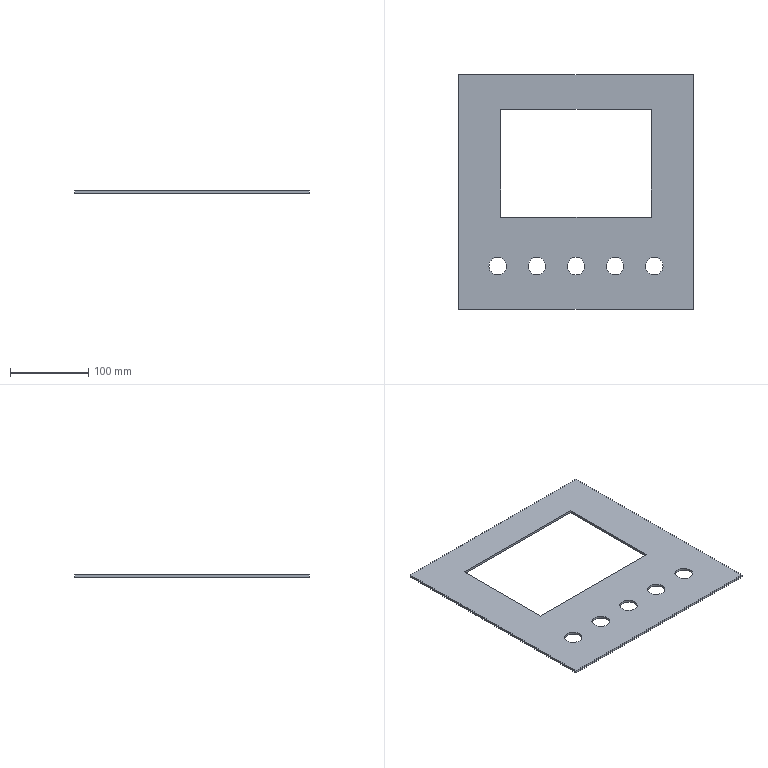Part | SolidWorks | features BaseBody 1 | 1 solid | 20 faces | box 300 x 300 x 3 mm | volume 184548 mm3 | cylinder 10 | plane 10 | commonest cylinder face diameters 22.5 x10
STEP:
#1=CARTESIAN_POINT('',(238.75,55.231,3.));
#2=VERTEX_POINT('',#1);
#3=CARTESIAN_POINT('',(261.25,55.231,3.));
#4=VERTEX_POINT('',#3);
#5=CARTESIAN_POINT('',(250.,55.231,3.));
#6=DIRECTION('',(0.,0.,1.));
#7=DIRECTION('',(-1.,0.,0.));
#8=AXIS2_PLACEMENT_3D('',#5,#6,#7);
#9=CIRCLE('',#8,11.25);
#10=EDGE_CURVE('',#2,#4,#9,.T.);
#11=ORIENTED_EDGE('',*,*,#10,.T.);
#12=CARTESIAN_POINT('',(261.25,55.231,0.));
#13=VERTEX_POINT('',#12);
#14=CARTESIAN_POINT('',(261.25,55.231,3.));
#15=DIRECTION('',(0.,0.,-1.));
#16=VECTOR('',#15,1000.);
#17=LINE('',#14,#16);
#18=EDGE_CURVE('',#4,#13,#17,.T.);
#19=ORIENTED_EDGE('',*,*,#18,.T.);
#20=CARTESIAN_POINT('',(238.75,55.231,0.));
#21=VERTEX_POINT('',#20);
#22=CARTESIAN_POINT('',(250.,55.231,0.));
#23=DIRECTION('',(0.,0.,1.));
#24=DIRECTION('',(-1.,0.,0.));
#25=AXIS2_PLACEMENT_3D('',#22,#23,#24);
#26=CIRCLE('',#25,11.25);
#27=EDGE_CURVE('',#21,#13,#26,.T.);
#28=ORIENTED_EDGE('',*,*,#27,.F.);
#29=CARTESIAN_POINT('',(238.75,55.231,3.));
#30=DIRECTION('',(0.,0.,-1.));
#31=VECTOR('',#30,1000.);
#32=LINE('',#29,#31);
#33=EDGE_CURVE('',#2,#21,#32,.T.);
#34=ORIENTED_EDGE('',*,*,#33,.F.);
#35=EDGE_LOOP('',(#11,#19,#28,#34));
#36=FACE_OUTER_BOUND('',#35,.T.);
#37=CARTESIAN_POINT('',(250.,55.231,3.));
#38=DIRECTION('',(0.,0.,-1.));
#39=DIRECTION('',(-1.,0.,0.));
#40=AXIS2_PLACEMENT_3D('',#37,#38,#39);
#41=CYLINDRICAL_SURFACE('',#40,11.25);
#42=ADVANCED_FACE('',(#36),#41,.F.);
#43=CARTESIAN_POINT('',(188.75,55.231,3.));
#44=VERTEX_POINT('',#43);
#45=CARTESIAN_POINT('',(211.25,55.231,3.));
#46=VERTEX_POINT('',#45);
#47=CARTESIAN_POINT('',(200.,55.231,3.));
#48=DIRECTION('',(0.,0.,1.));
#49=DIRECTION('',(-1.,0.,0.));
#50=AXIS2_PLACEMENT_3D('',#47,#48,#49);
#51=CIRCLE('',#50,11.25);
#52=EDGE_CURVE('',#44,#46,#51,.T.);
#53=ORIENTED_EDGE('',*,*,#52,.T.);
#54=CARTESIAN_POINT('',(211.25,55.231,0.));
#55=VERTEX_POINT('',#54);
#56=CARTESIAN_POINT('',(211.25,55.231,3.));
#57=DIRECTION('',(0.,0.,-1.));
#58=VECTOR('',#57,1000.);
#59=LINE('',#56,#58);
#60=EDGE_CURVE('',#46,#55,#59,.T.);
#61=ORIENTED_EDGE('',*,*,#60,.T.);
#62=CARTESIAN_POINT('',(188.75,55.231,0.));
#63=VERTEX_POINT('',#62);
#64=CARTESIAN_POINT('',(200.,55.231,0.));
#65=DIRECTION('',(0.,0.,1.));
#66=DIRECTION('',(-1.,0.,0.));
#67=AXIS2_PLACEMENT_3D('',#64,#65,#66);
#68=CIRCLE('',#67,11.25);
#69=EDGE_CURVE('',#63,#55,#68,.T.);
#70=ORIENTED_EDGE('',*,*,#69,.F.);
#71=CARTESIAN_POINT('',(188.75,55.231,3.));
#72=DIRECTION('',(0.,0.,-1.));
#73=VECTOR('',#72,1000.);
#74=LINE('',#71,#73);
#75=EDGE_CURVE('',#44,#63,#74,.T.);
#76=ORIENTED_EDGE('',*,*,#75,.F.);
#77=EDGE_LOOP('',(#53,#61,#70,#76));
#78=FACE_OUTER_BOUND('',#77,.T.);
#79=CARTESIAN_POINT('',(200.,55.231,3.));
#80=DIRECTION('',(0.,0.,-1.));
#81=DIRECTION('',(-1.,0.,0.));
#82=AXIS2_PLACEMENT_3D('',#79,#80,#81);
#83=CYLINDRICAL_SURFACE('',#82,11.25);
#84=ADVANCED_FACE('',(#78),#83,.F.);
#85=CARTESIAN_POINT('',(138.75,55.231,3.));
#86=VERTEX_POINT('',#85);
#87=CARTESIAN_POINT('',(161.25,55.231,3.));
#88=VERTEX_POINT('',#87);
#89=CARTESIAN_POINT('',(150.,55.231,3.));
#90=DIRECTION('',(0.,0.,1.));
#91=DIRECTION('',(-1.,0.,0.));
#92=AXIS2_PLACEMENT_3D('',#89,#90,#91);
#93=CIRCLE('',#92,11.25);
#94=EDGE_CURVE('',#86,#88,#93,.T.);
#95=ORIENTED_EDGE('',*,*,#94,.T.);
#96=CARTESIAN_POINT('',(161.25,55.231,0.));
#97=VERTEX_POINT('',#96);
#98=CARTESIAN_POINT('',(161.25,55.231,3.));
#99=DIRECTION('',(0.,0.,-1.));
#100=VECTOR('',#99,1000.);
#101=LINE('',#98,#100);
#102=EDGE_CURVE('',#88,#97,#101,.T.);
#103=ORIENTED_EDGE('',*,*,#102,.T.);
#104=CARTESIAN_POINT('',(138.75,55.231,0.));
#105=VERTEX_POINT('',#104);
#106=CARTESIAN_POINT('',(150.,55.231,0.));
#107=DIRECTION('',(0.,0.,1.));
#108=DIRECTION('',(-1.,0.,0.));
#109=AXIS2_PLACEMENT_3D('',#106,#107,#108);
#110=CIRCLE('',#109,11.25);
#111=EDGE_CURVE('',#105,#97,#110,.T.);
#112=ORIENTED_EDGE('',*,*,#111,.F.);
#113=CARTESIAN_POINT('',(138.75,55.231,3.));
#114=DIRECTION('',(0.,0.,-1.));
#115=VECTOR('',#114,1000.);
#116=LINE('',#113,#115);
#117=EDGE_CURVE('',#86,#105,#116,.T.);
#118=ORIENTED_EDGE('',*,*,#117,.F.);
#119=EDGE_LOOP('',(#95,#103,#112,#118));
#120=FACE_OUTER_BOUND('',#119,.T.);
#121=CARTESIAN_POINT('',(150.,55.231,3.));
#122=DIRECTION('',(0.,0.,-1.));
#123=DIRECTION('',(-1.,0.,0.));
#124=AXIS2_PLACEMENT_3D('',#121,#122,#123);
#125=CYLINDRICAL_SURFACE('',#124,11.25);
#126=ADVANCED_FACE('',(#120),#125,.F.);
#127=CARTESIAN_POINT('',(88.75,55.231,3.));
#128=VERTEX_POINT('',#127);
#129=CARTESIAN_POINT('',(111.25,55.231,3.));
#130=VERTEX_POINT('',#129);
#131=CARTESIAN_POINT('',(100.,55.231,3.));
#132=DIRECTION('',(0.,0.,1.));
#133=DIRECTION('',(-1.,0.,0.));
#134=AXIS2_PLACEMENT_3D('',#131,#132,#133);
#135=CIRCLE('',#134,11.25);
#136=EDGE_CURVE('',#128,#130,#135,.T.);
#137=ORIENTED_EDGE('',*,*,#136,.T.);
#138=CARTESIAN_POINT('',(111.25,55.231,0.));
#139=VERTEX_POINT('',#138);
#140=CARTESIAN_POINT('',(111.25,55.231,3.));
#141=DIRECTION('',(0.,0.,-1.));
#142=VECTOR('',#141,1000.);
#143=LINE('',#140,#142);
#144=EDGE_CURVE('',#130,#139,#143,.T.);
#145=ORIENTED_EDGE('',*,*,#144,.T.);
#146=CARTESIAN_POINT('',(88.75,55.231,0.));
#147=VERTEX_POINT('',#146);
#148=CARTESIAN_POINT('',(100.,55.231,0.));
#149=DIRECTION('',(0.,0.,1.));
#150=DIRECTION('',(-1.,0.,0.));
#151=AXIS2_PLACEMENT_3D('',#148,#149,#150);
#152=CIRCLE('',#151,11.25);
#153=EDGE_CURVE('',#147,#139,#152,.T.);
#154=ORIENTED_EDGE('',*,*,#153,.F.);
#155=CARTESIAN_POINT('',(88.75,55.231,3.));
#156=DIRECTION('',(0.,0.,-1.));
#157=VECTOR('',#156,1000.);
#158=LINE('',#155,#157);
#159=EDGE_CURVE('',#128,#147,#158,.T.);
#160=ORIENTED_EDGE('',*,*,#159,.F.);
#161=EDGE_LOOP('',(#137,#145,#154,#160));
#162=FACE_OUTER_BOUND('',#161,.T.);
#163=CARTESIAN_POINT('',(100.,55.231,3.));
#164=DIRECTION('',(0.,0.,-1.));
#165=DIRECTION('',(-1.,0.,0.));
#166=AXIS2_PLACEMENT_3D('',#163,#164,#165);
#167=CYLINDRICAL_SURFACE('',#166,11.25);
#168=ADVANCED_FACE('',(#162),#167,.F.);
#169=CARTESIAN_POINT('',(38.75,55.231,3.));
#170=VERTEX_POINT('',#169);
#171=CARTESIAN_POINT('',(61.25,55.231,3.));
#172=VERTEX_POINT('',#171);
#173=CARTESIAN_POINT('',(50.,55.231,3.));
#174=DIRECTION('',(0.,0.,1.));
#175=DIRECTION('',(-1.,0.,0.));
#176=AXIS2_PLACEMENT_3D('',#173,#174,#175);
#177=CIRCLE('',#176,11.25);
#178=EDGE_CURVE('',#170,#172,#177,.T.);
#179=ORIENTED_EDGE('',*,*,#178,.T.);
#180=CARTESIAN_POINT('',(61.25,55.231,0.));
#181=VERTEX_POINT('',#180);
#182=CARTESIAN_POINT('',(61.25,55.231,3.));
#183=DIRECTION('',(0.,0.,-1.));
#184=VECTOR('',#183,1000.);
#185=LINE('',#182,#184);
#186=EDGE_CURVE('',#172,#181,#185,.T.);
#187=ORIENTED_EDGE('',*,*,#186,.T.);
#188=CARTESIAN_POINT('',(38.75,55.231,0.));
#189=VERTEX_POINT('',#188);
#190=CARTESIAN_POINT('',(50.,55.231,0.));
#191=DIRECTION('',(0.,0.,1.));
#192=DIRECTION('',(-1.,0.,0.));
#193=AXIS2_PLACEMENT_3D('',#190,#191,#192);
#194=CIRCLE('',#193,11.25);
#195=EDGE_CURVE('',#189,#181,#194,.T.);
#196=ORIENTED_EDGE('',*,*,#195,.F.);
#197=CARTESIAN_POINT('',(38.75,55.231,3.));
#198=DIRECTION('',(0.,0.,-1.));
#199=VECTOR('',#198,1000.);
#200=LINE('',#197,#199);
#201=EDGE_CURVE('',#170,#189,#200,.T.);
#202=ORIENTED_EDGE('',*,*,#201,.F.);
#203=EDGE_LOOP('',(#179,#187,#196,#202));
#204=FACE_OUTER_BOUND('',#203,.T.);
#205=CARTESIAN_POINT('',(50.,55.231,3.));
#206=DIRECTION('',(0.,0.,-1.));
#207=DIRECTION('',(-1.,0.,0.));
#208=AXIS2_PLACEMENT_3D('',#205,#206,#207);
#209=CYLINDRICAL_SURFACE('',#208,11.25);
#210=ADVANCED_FACE('',(#204),#209,.F.);
#211=ORIENTED_EDGE('',*,*,#10,.F.);
#212=CARTESIAN_POINT('',(250.,55.231,3.));
#213=DIRECTION('',(0.,0.,1.));
#214=DIRECTION('',(-1.,0.,0.));
#215=AXIS2_PLACEMENT_3D('',#212,#213,#214);
#216=CIRCLE('',#215,11.25);
#217=EDGE_CURVE('',#4,#2,#216,.T.);
#218=ORIENTED_EDGE('',*,*,#217,.F.);
#219=EDGE_LOOP('',(#211,#218));
#220=FACE_BOUND('',#219,.T.);
#221=ORIENTED_EDGE('',*,*,#52,.F.);
#222=CARTESIAN_POINT('',(200.,55.231,3.));
#223=DIRECTION('',(0.,0.,1.));
#224=DIRECTION('',(-1.,0.,0.));
#225=AXIS2_PLACEMENT_3D('',#222,#223,#224);
#226=CIRCLE('',#225,11.25);
#227=EDGE_CURVE('',#46,#44,#226,.T.);
#228=ORIENTED_EDGE('',*,*,#227,.F.);
#229=EDGE_LOOP('',(#221,#228));
#230=FACE_BOUND('',#229,.T.);
#231=ORIENTED_EDGE('',*,*,#94,.F.);
#232=CARTESIAN_POINT('',(150.,55.231,3.));
#233=DIRECTION('',(0.,0.,1.));
#234=DIRECTION('',(-1.,0.,0.));
#235=AXIS2_PLACEMENT_3D('',#232,#233,#234);
#236=CIRCLE('',#235,11.25);
#237=EDGE_CURVE('',#88,#86,#236,.T.);
#238=ORIENTED_EDGE('',*,*,#237,.F.);
#239=EDGE_LOOP('',(#231,#238));
#240=FACE_BOUND('',#239,.T.);
#241=ORIENTED_EDGE('',*,*,#136,.F.);
#242=CARTESIAN_POINT('',(100.,55.231,3.));
#243=DIRECTION('',(0.,0.,1.));
#244=DIRECTION('',(-1.,0.,0.));
#245=AXIS2_PLACEMENT_3D('',#242,#243,#244);
#246=CIRCLE('',#245,11.25);
#247=EDGE_CURVE('',#130,#128,#246,.T.);
#248=ORIENTED_EDGE('',*,*,#247,.F.);
#249=EDGE_LOOP('',(#241,#248));
#250=FACE_BOUND('',#249,.T.);
#251=ORIENTED_EDGE('',*,*,#178,.F.);
#252=CARTESIAN_POINT('',(50.,55.231,3.));
#253=DIRECTION('',(0.,0.,1.));
#254=DIRECTION('',(-1.,0.,0.));
#255=AXIS2_PLACEMENT_3D('',#252,#253,#254);
#256=CIRCLE('',#255,11.25);
#257=EDGE_CURVE('',#172,#170,#256,.T.);
#258=ORIENTED_EDGE('',*,*,#257,.F.);
#259=EDGE_LOOP('',(#251,#258));
#260=FACE_BOUND('',#259,.T.);
#261=CARTESIAN_POINT('',(54.,117.73,3.));
#262=VERTEX_POINT('',#261);
#263=CARTESIAN_POINT('',(246.,117.73,3.));
#264=VERTEX_POINT('',#263);
#265=CARTESIAN_POINT('',(0.,117.73,3.));
#266=DIRECTION('',(1.,0.,0.));
#267=VECTOR('',#266,1000.);
#268=LINE('',#265,#267);
#269=EDGE_CURVE('',#262,#264,#268,.T.);
#270=ORIENTED_EDGE('',*,*,#269,.F.);
#271=CARTESIAN_POINT('',(54.,255.73,3.));
#272=VERTEX_POINT('',#271);
#273=CARTESIAN_POINT('',(54.,0.,3.));
#274=DIRECTION('',(0.,-1.,0.));
#275=VECTOR('',#274,1000.);
#276=LINE('',#273,#275);
#277=EDGE_CURVE('',#272,#262,#276,.T.);
#278=ORIENTED_EDGE('',*,*,#277,.F.);
#279=CARTESIAN_POINT('',(246.,255.73,3.));
#280=VERTEX_POINT('',#279);
#281=CARTESIAN_POINT('',(0.,255.73,3.));
#282=DIRECTION('',(-1.,0.,0.));
#283=VECTOR('',#282,1000.);
#284=LINE('',#281,#283);
#285=EDGE_CURVE('',#280,#272,#284,.T.);
#286=ORIENTED_EDGE('',*,*,#285,.F.);
#287=CARTESIAN_POINT('',(246.,0.,3.));
#288=DIRECTION('',(0.,1.,0.));
#289=VECTOR('',#288,1000.);
#290=LINE('',#287,#289);
#291=EDGE_CURVE('',#264,#280,#290,.T.);
#292=ORIENTED_EDGE('',*,*,#291,.F.);
#293=EDGE_LOOP('',(#270,#278,#286,#292));
#294=FACE_BOUND('',#293,.T.);
#295=CARTESIAN_POINT('',(300.,0.,3.));
#296=VERTEX_POINT('',#295);
#297=CARTESIAN_POINT('',(0.,0.,3.));
#298=VERTEX_POINT('',#297);
#299=CARTESIAN_POINT('',(0.,0.,3.));
#300=DIRECTION('',(-1.,0.,0.));
#301=VECTOR('',#300,1000.);
#302=LINE('',#299,#301);
#303=EDGE_CURVE('',#296,#298,#302,.T.);
#304=ORIENTED_EDGE('',*,*,#303,.F.);
#305=CARTESIAN_POINT('',(300.,300.,3.));
#306=VERTEX_POINT('',#305);
#307=CARTESIAN_POINT('',(300.,0.,3.));
#308=DIRECTION('',(0.,-1.,0.));
#309=VECTOR('',#308,1000.);
#310=LINE('',#307,#309);
#311=EDGE_CURVE('',#306,#296,#310,.T.);
#312=ORIENTED_EDGE('',*,*,#311,.F.);
#313=CARTESIAN_POINT('',(0.,300.,3.));
#314=VERTEX_POINT('',#313);
#315=CARTESIAN_POINT('',(0.,300.,3.));
#316=DIRECTION('',(1.,0.,0.));
#317=VECTOR('',#316,1000.);
#318=LINE('',#315,#317);
#319=EDGE_CURVE('',#314,#306,#318,.T.);
#320=ORIENTED_EDGE('',*,*,#319,.F.);
#321=CARTESIAN_POINT('',(0.,0.,3.));
#322=DIRECTION('',(0.,1.,0.));
#323=VECTOR('',#322,1000.);
#324=LINE('',#321,#323);
#325=EDGE_CURVE('',#298,#314,#324,.T.);
#326=ORIENTED_EDGE('',*,*,#325,.F.);
#327=EDGE_LOOP('',(#304,#312,#320,#326));
#328=FACE_OUTER_BOUND('',#327,.T.);
#329=CARTESIAN_POINT('',(0.,0.,3.));
#330=DIRECTION('',(0.,0.,-1.));
#331=DIRECTION('',(-1.,0.,0.));
#332=AXIS2_PLACEMENT_3D('',#329,#330,#331);
#333=PLANE('',#332);
#334=ADVANCED_FACE('',(#220,#230,#240,#250,#260,#294,#328),#333,.F.);
#335=ORIENTED_EDGE('',*,*,#18,.F.);
#336=ORIENTED_EDGE('',*,*,#217,.T.);
#337=ORIENTED_EDGE('',*,*,#33,.T.);
#338=CARTESIAN_POINT('',(250.,55.231,0.));
#339=DIRECTION('',(0.,0.,1.));
#340=DIRECTION('',(-1.,0.,0.));
#341=AXIS2_PLACEMENT_3D('',#338,#339,#340);
#342=CIRCLE('',#341,11.25);
#343=EDGE_CURVE('',#13,#21,#342,.T.);
#344=ORIENTED_EDGE('',*,*,#343,.F.);
#345=EDGE_LOOP('',(#335,#336,#337,#344));
#346=FACE_OUTER_BOUND('',#345,.T.);
#347=CARTESIAN_POINT('',(250.,55.231,3.));
#348=DIRECTION('',(0.,0.,-1.));
#349=DIRECTION('',(-1.,0.,0.));
#350=AXIS2_PLACEMENT_3D('',#347,#348,#349);
#351=CYLINDRICAL_SURFACE('',#350,11.25);
#352=ADVANCED_FACE('',(#346),#351,.F.);
#353=ORIENTED_EDGE('',*,*,#60,.F.);
#354=ORIENTED_EDGE('',*,*,#227,.T.);
#355=ORIENTED_EDGE('',*,*,#75,.T.);
#356=CARTESIAN_POINT('',(200.,55.231,0.));
#357=DIRECTION('',(0.,0.,1.));
#358=DIRECTION('',(-1.,0.,0.));
#359=AXIS2_PLACEMENT_3D('',#356,#357,#358);
#360=CIRCLE('',#359,11.25);
#361=EDGE_CURVE('',#55,#63,#360,.T.);
#362=ORIENTED_EDGE('',*,*,#361,.F.);
#363=EDGE_LOOP('',(#353,#354,#355,#362));
#364=FACE_OUTER_BOUND('',#363,.T.);
#365=CARTESIAN_POINT('',(200.,55.231,3.));
#366=DIRECTION('',(0.,0.,-1.));
#367=DIRECTION('',(-1.,0.,0.));
#368=AXIS2_PLACEMENT_3D('',#365,#366,#367);
#369=CYLINDRICAL_SURFACE('',#368,11.25);
#370=ADVANCED_FACE('',(#364),#369,.F.);
#371=ORIENTED_EDGE('',*,*,#102,.F.);
#372=ORIENTED_EDGE('',*,*,#237,.T.);
#373=ORIENTED_EDGE('',*,*,#117,.T.);
#374=CARTESIAN_POINT('',(150.,55.231,0.));
#375=DIRECTION('',(0.,0.,1.));
#376=DIRECTION('',(-1.,0.,0.));
#377=AXIS2_PLACEMENT_3D('',#374,#375,#376);
#378=CIRCLE('',#377,11.25);
#379=EDGE_CURVE('',#97,#105,#378,.T.);
#380=ORIENTED_EDGE('',*,*,#379,.F.);
#381=EDGE_LOOP('',(#371,#372,#373,#380));
#382=FACE_OUTER_BOUND('',#381,.T.);
#383=CARTESIAN_POINT('',(150.,55.231,3.));
#384=DIRECTION('',(0.,0.,-1.));
#385=DIRECTION('',(-1.,0.,0.));
#386=AXIS2_PLACEMENT_3D('',#383,#384,#385);
#387=CYLINDRICAL_SURFACE('',#386,11.25);
#388=ADVANCED_FACE('',(#382),#387,.F.);
#389=ORIENTED_EDGE('',*,*,#144,.F.);
#390=ORIENTED_EDGE('',*,*,#247,.T.);
#391=ORIENTED_EDGE('',*,*,#159,.T.);
#392=CARTESIAN_POINT('',(100.,55.231,0.));
#393=DIRECTION('',(0.,0.,1.));
#394=DIRECTION('',(-1.,0.,0.));
#395=AXIS2_PLACEMENT_3D('',#392,#393,#394);
#396=CIRCLE('',#395,11.25);
#397=EDGE_CURVE('',#139,#147,#396,.T.);
#398=ORIENTED_EDGE('',*,*,#397,.F.);
#399=EDGE_LOOP('',(#389,#390,#391,#398));
#400=FACE_OUTER_BOUND('',#399,.T.);
#401=CARTESIAN_POINT('',(100.,55.231,3.));
#402=DIRECTION('',(0.,0.,-1.));
#403=DIRECTION('',(-1.,0.,0.));
#404=AXIS2_PLACEMENT_3D('',#401,#402,#403);
#405=CYLINDRICAL_SURFACE('',#404,11.25);
#406=ADVANCED_FACE('',(#400),#405,.F.);
#407=ORIENTED_EDGE('',*,*,#186,.F.);
#408=ORIENTED_EDGE('',*,*,#257,.T.);
#409=ORIENTED_EDGE('',*,*,#201,.T.);
#410=CARTESIAN_POINT('',(50.,55.231,0.));
#411=DIRECTION('',(0.,0.,1.));
#412=DIRECTION('',(-1.,0.,0.));
#413=AXIS2_PLACEMENT_3D('',#410,#411,#412);
#414=CIRCLE('',#413,11.25);
#415=EDGE_CURVE('',#181,#189,#414,.T.);
#416=ORIENTED_EDGE('',*,*,#415,.F.);
#417=EDGE_LOOP('',(#407,#408,#409,#416));
#418=FACE_OUTER_BOUND('',#417,.T.);
#419=CARTESIAN_POINT('',(50.,55.231,3.));
#420=DIRECTION('',(0.,0.,-1.));
#421=DIRECTION('',(-1.,0.,0.));
#422=AXIS2_PLACEMENT_3D('',#419,#420,#421);
#423=CYLINDRICAL_SURFACE('',#422,11.25);
#424=ADVANCED_FACE('',(#418),#423,.F.);
#425=ORIENTED_EDGE('',*,*,#291,.T.);
#426=CARTESIAN_POINT('',(246.,255.73,0.));
#427=VERTEX_POINT('',#426);
#428=CARTESIAN_POINT('',(246.,255.73,3.));
#429=DIRECTION('',(0.,0.,-1.));
#430=VECTOR('',#429,1000.);
#431=LINE('',#428,#430);
#432=EDGE_CURVE('',#280,#427,#431,.T.);
#433=ORIENTED_EDGE('',*,*,#432,.T.);
#434=CARTESIAN_POINT('',(246.,117.73,0.));
#435=VERTEX_POINT('',#434);
#436=CARTESIAN_POINT('',(246.,255.73,0.));
#437=DIRECTION('',(0.,-1.,0.));
#438=VECTOR('',#437,1000.);
#439=LINE('',#436,#438);
#440=EDGE_CURVE('',#427,#435,#439,.T.);
#441=ORIENTED_EDGE('',*,*,#440,.T.);
#442=CARTESIAN_POINT('',(246.,117.73,3.));
#443=DIRECTION('',(0.,0.,1.));
#444=VECTOR('',#443,1000.);
#445=LINE('',#442,#444);
#446=EDGE_CURVE('',#435,#264,#445,.T.);
#447=ORIENTED_EDGE('',*,*,#446,.T.);
#448=EDGE_LOOP('',(#425,#433,#441,#447));
#449=FACE_OUTER_BOUND('',#448,.T.);
#450=CARTESIAN_POINT('',(246.,255.73,3.));
#451=DIRECTION('',(-1.,0.,0.));
#452=DIRECTION('',(0.,0.,1.));
#453=AXIS2_PLACEMENT_3D('',#450,#451,#452);
#454=PLANE('',#453);
#455=ADVANCED_FACE('',(#449),#454,.T.);
#456=ORIENTED_EDGE('',*,*,#269,.T.);
#457=ORIENTED_EDGE('',*,*,#446,.F.);
#458=CARTESIAN_POINT('',(54.,117.73,0.));
#459=VERTEX_POINT('',#458);
#460=CARTESIAN_POINT('',(54.,117.73,0.));
#461=DIRECTION('',(-1.,0.,0.));
#462=VECTOR('',#461,1000.);
#463=LINE('',#460,#462);
#464=EDGE_CURVE('',#435,#459,#463,.T.);
#465=ORIENTED_EDGE('',*,*,#464,.T.);
#466=CARTESIAN_POINT('',(54.,117.73,3.));
#467=DIRECTION('',(0.,0.,1.));
#468=VECTOR('',#467,1000.);
#469=LINE('',#466,#468);
#470=EDGE_CURVE('',#459,#262,#469,.T.);
#471=ORIENTED_EDGE('',*,*,#470,.T.);
#472=EDGE_LOOP('',(#456,#457,#465,#471));
#473=FACE_OUTER_BOUND('',#472,.T.);
#474=CARTESIAN_POINT('',(54.,117.73,3.));
#475=DIRECTION('',(0.,1.,0.));
#476=DIRECTION('',(0.,0.,1.));
#477=AXIS2_PLACEMENT_3D('',#474,#475,#476);
#478=PLANE('',#477);
#479=ADVANCED_FACE('',(#473),#478,.T.);
#480=ORIENTED_EDGE('',*,*,#277,.T.);
#481=ORIENTED_EDGE('',*,*,#470,.F.);
#482=CARTESIAN_POINT('',(54.,255.73,0.));
#483=VERTEX_POINT('',#482);
#484=CARTESIAN_POINT('',(54.,255.73,0.));
#485=DIRECTION('',(0.,1.,0.));
#486=VECTOR('',#485,1000.);
#487=LINE('',#484,#486);
#488=EDGE_CURVE('',#459,#483,#487,.T.);
#489=ORIENTED_EDGE('',*,*,#488,.T.);
#490=CARTESIAN_POINT('',(54.,255.73,3.));
#491=DIRECTION('',(0.,0.,1.));
#492=VECTOR('',#491,1000.);
#493=LINE('',#490,#492);
#494=EDGE_CURVE('',#483,#272,#493,.T.);
#495=ORIENTED_EDGE('',*,*,#494,.T.);
#496=EDGE_LOOP('',(#480,#481,#489,#495));
#497=FACE_OUTER_BOUND('',#496,.T.);
#498=CARTESIAN_POINT('',(54.,255.73,3.));
#499=DIRECTION('',(1.,0.,0.));
#500=DIRECTION('',(0.,0.,-1.));
#501=AXIS2_PLACEMENT_3D('',#498,#499,#500);
#502=PLANE('',#501);
#503=ADVANCED_FACE('',(#497),#502,.T.);
#504=ORIENTED_EDGE('',*,*,#285,.T.);
#505=ORIENTED_EDGE('',*,*,#494,.F.);
#506=CARTESIAN_POINT('',(54.,255.73,0.));
#507=DIRECTION('',(1.,0.,0.));
#508=VECTOR('',#507,1000.);
#509=LINE('',#506,#508);
#510=EDGE_CURVE('',#483,#427,#509,.T.);
#511=ORIENTED_EDGE('',*,*,#510,.T.);
#512=ORIENTED_EDGE('',*,*,#432,.F.);
#513=EDGE_LOOP('',(#504,#505,#511,#512));
#514=FACE_OUTER_BOUND('',#513,.T.);
#515=CARTESIAN_POINT('',(54.,255.73,3.));
#516=DIRECTION('',(0.,-1.,0.));
#517=DIRECTION('',(1.,0.,0.));
#518=AXIS2_PLACEMENT_3D('',#515,#516,#517);
#519=PLANE('',#518);
#520=ADVANCED_FACE('',(#514),#519,.T.);
#521=CARTESIAN_POINT('',(0.,0.,0.));
#522=VERTEX_POINT('',#521);
#523=CARTESIAN_POINT('',(0.,0.,3.));
#524=DIRECTION('',(0.,0.,-1.));
#525=VECTOR('',#524,1000.);
#526=LINE('',#523,#525);
#527=EDGE_CURVE('',#298,#522,#526,.T.);
#528=ORIENTED_EDGE('',*,*,#527,.F.);
#529=ORIENTED_EDGE('',*,*,#325,.T.);
#530=CARTESIAN_POINT('',(0.,300.,0.));
#531=VERTEX_POINT('',#530);
#532=CARTESIAN_POINT('',(0.,300.,3.));
#533=DIRECTION('',(0.,0.,1.));
#534=VECTOR('',#533,1000.);
#535=LINE('',#532,#534);
#536=EDGE_CURVE('',#531,#314,#535,.T.);
#537=ORIENTED_EDGE('',*,*,#536,.F.);
#538=CARTESIAN_POINT('',(0.,0.,0.));
#539=DIRECTION('',(0.,1.,0.));
#540=VECTOR('',#539,1000.);
#541=LINE('',#538,#540);
#542=EDGE_CURVE('',#522,#531,#541,.T.);
#543=ORIENTED_EDGE('',*,*,#542,.F.);
#544=EDGE_LOOP('',(#528,#529,#537,#543));
#545=FACE_OUTER_BOUND('',#544,.T.);
#546=CARTESIAN_POINT('',(0.,0.,3.));
#547=DIRECTION('',(1.,0.,0.));
#548=DIRECTION('',(0.,0.,-1.));
#549=AXIS2_PLACEMENT_3D('',#546,#547,#548);
#550=PLANE('',#549);
#551=ADVANCED_FACE('',(#545),#550,.F.);
#552=CARTESIAN_POINT('',(300.,0.,0.));
#553=VERTEX_POINT('',#552);
#554=CARTESIAN_POINT('',(300.,0.,3.));
#555=DIRECTION('',(0.,0.,-1.));
#556=VECTOR('',#555,1000.);
#557=LINE('',#554,#556);
#558=EDGE_CURVE('',#296,#553,#557,.T.);
#559=ORIENTED_EDGE('',*,*,#558,.F.);
#560=ORIENTED_EDGE('',*,*,#303,.T.);
#561=ORIENTED_EDGE('',*,*,#527,.T.);
#562=CARTESIAN_POINT('',(0.,0.,0.));
#563=DIRECTION('',(-1.,0.,0.));
#564=VECTOR('',#563,1000.);
#565=LINE('',#562,#564);
#566=EDGE_CURVE('',#553,#522,#565,.T.);
#567=ORIENTED_EDGE('',*,*,#566,.F.);
#568=EDGE_LOOP('',(#559,#560,#561,#567));
#569=FACE_OUTER_BOUND('',#568,.T.);
#570=CARTESIAN_POINT('',(0.,0.,3.));
#571=DIRECTION('',(0.,1.,0.));
#572=DIRECTION('',(0.,0.,1.));
#573=AXIS2_PLACEMENT_3D('',#570,#571,#572);
#574=PLANE('',#573);
#575=ADVANCED_FACE('',(#569),#574,.F.);
#576=CARTESIAN_POINT('',(300.,300.,0.));
#577=VERTEX_POINT('',#576);
#578=CARTESIAN_POINT('',(300.,300.,3.));
#579=DIRECTION('',(0.,0.,-1.));
#580=VECTOR('',#579,1000.);
#581=LINE('',#578,#580);
#582=EDGE_CURVE('',#306,#577,#581,.T.);
#583=ORIENTED_EDGE('',*,*,#582,.F.);
#584=ORIENTED_EDGE('',*,*,#311,.T.);
#585=ORIENTED_EDGE('',*,*,#558,.T.);
#586=CARTESIAN_POINT('',(300.,0.,0.));
#587=DIRECTION('',(0.,-1.,0.));
#588=VECTOR('',#587,1000.);
#589=LINE('',#586,#588);
#590=EDGE_CURVE('',#577,#553,#589,.T.);
#591=ORIENTED_EDGE('',*,*,#590,.F.);
#592=EDGE_LOOP('',(#583,#584,#585,#591));
#593=FACE_OUTER_BOUND('',#592,.T.);
#594=CARTESIAN_POINT('',(300.,0.,3.));
#595=DIRECTION('',(-1.,0.,0.));
#596=DIRECTION('',(0.,0.,1.));
#597=AXIS2_PLACEMENT_3D('',#594,#595,#596);
#598=PLANE('',#597);
#599=ADVANCED_FACE('',(#593),#598,.F.);
#600=ORIENTED_EDGE('',*,*,#536,.T.);
#601=ORIENTED_EDGE('',*,*,#319,.T.);
#602=ORIENTED_EDGE('',*,*,#582,.T.);
#603=CARTESIAN_POINT('',(0.,300.,0.));
#604=DIRECTION('',(1.,0.,0.));
#605=VECTOR('',#604,1000.);
#606=LINE('',#603,#605);
#607=EDGE_CURVE('',#531,#577,#606,.T.);
#608=ORIENTED_EDGE('',*,*,#607,.F.);
#609=EDGE_LOOP('',(#600,#601,#602,#608));
#610=FACE_OUTER_BOUND('',#609,.T.);
#611=CARTESIAN_POINT('',(0.,300.,3.));
#612=DIRECTION('',(0.,-1.,0.));
#613=DIRECTION('',(0.,0.,-1.));
#614=AXIS2_PLACEMENT_3D('',#611,#612,#613);
#615=PLANE('',#614);
#616=ADVANCED_FACE('',(#610),#615,.F.);
#617=ORIENTED_EDGE('',*,*,#27,.T.);
#618=ORIENTED_EDGE('',*,*,#343,.T.);
#619=EDGE_LOOP('',(#617,#618));
#620=FACE_BOUND('',#619,.T.);
#621=ORIENTED_EDGE('',*,*,#111,.T.);
#622=ORIENTED_EDGE('',*,*,#379,.T.);
#623=EDGE_LOOP('',(#621,#622));
#624=FACE_BOUND('',#623,.T.);
#625=ORIENTED_EDGE('',*,*,#195,.T.);
#626=ORIENTED_EDGE('',*,*,#415,.T.);
#627=EDGE_LOOP('',(#625,#626));
#628=FACE_BOUND('',#627,.T.);
#629=ORIENTED_EDGE('',*,*,#590,.T.);
#630=ORIENTED_EDGE('',*,*,#566,.T.);
#631=ORIENTED_EDGE('',*,*,#542,.T.);
#632=ORIENTED_EDGE('',*,*,#607,.T.);
#633=EDGE_LOOP('',(#629,#630,#631,#632));
#634=FACE_OUTER_BOUND('',#633,.T.);
#635=ORIENTED_EDGE('',*,*,#510,.F.);
#636=ORIENTED_EDGE('',*,*,#488,.F.);
#637=ORIENTED_EDGE('',*,*,#464,.F.);
#638=ORIENTED_EDGE('',*,*,#440,.F.);
#639=EDGE_LOOP('',(#635,#636,#637,#638));
#640=FACE_BOUND('',#639,.T.);
#641=ORIENTED_EDGE('',*,*,#153,.T.);
#642=ORIENTED_EDGE('',*,*,#397,.T.);
#643=EDGE_LOOP('',(#641,#642));
#644=FACE_BOUND('',#643,.T.);
#645=ORIENTED_EDGE('',*,*,#69,.T.);
#646=ORIENTED_EDGE('',*,*,#361,.T.);
#647=EDGE_LOOP('',(#645,#646));
#648=FACE_BOUND('',#647,.T.);
#649=CARTESIAN_POINT('',(0.,0.,0.));
#650=DIRECTION('',(0.,0.,-1.));
#651=DIRECTION('',(-1.,0.,0.));
#652=AXIS2_PLACEMENT_3D('',#649,#650,#651);
#653=PLANE('',#652);
#654=ADVANCED_FACE('',(#620,#624,#628,#634,#640,#644,#648),#653,.T.);
#655=CLOSED_SHELL('',(#42,#84,#126,#168,#210,#334,#352,#370,#388,#406,#424,#455,#479,#503,#520,#551,#575,#599,#616,#654));
#656=MANIFOLD_SOLID_BREP('',#655);
#657=CARTESIAN_POINT('',(0.,0.,0.));
#658=DIRECTION('',(0.,0.,1.));
#659=DIRECTION('',(1.,0.,0.));
#660=AXIS2_PLACEMENT_3D('',#657,#658,#659);
#661=(LENGTH_UNIT()NAMED_UNIT(*)SI_UNIT(.MILLI.,.METRE.));
#662=UNCERTAINTY_MEASURE_WITH_UNIT(LENGTH_MEASURE(0.00001),#661,'','');
#663=(NAMED_UNIT(*)PLANE_ANGLE_UNIT()SI_UNIT($,.RADIAN.));
#664=(NAMED_UNIT(*)SI_UNIT($,.STERADIAN.)SOLID_ANGLE_UNIT());
#665=(GEOMETRIC_REPRESENTATION_CONTEXT(3)GLOBAL_UNCERTAINTY_ASSIGNED_CONTEXT((#662))GLOBAL_UNIT_ASSIGNED_CONTEXT((#661,#663,#664))REPRESENTATION_CONTEXT('',''));
#666=ADVANCED_BREP_SHAPE_REPRESENTATION('',(#656,#660),#665);